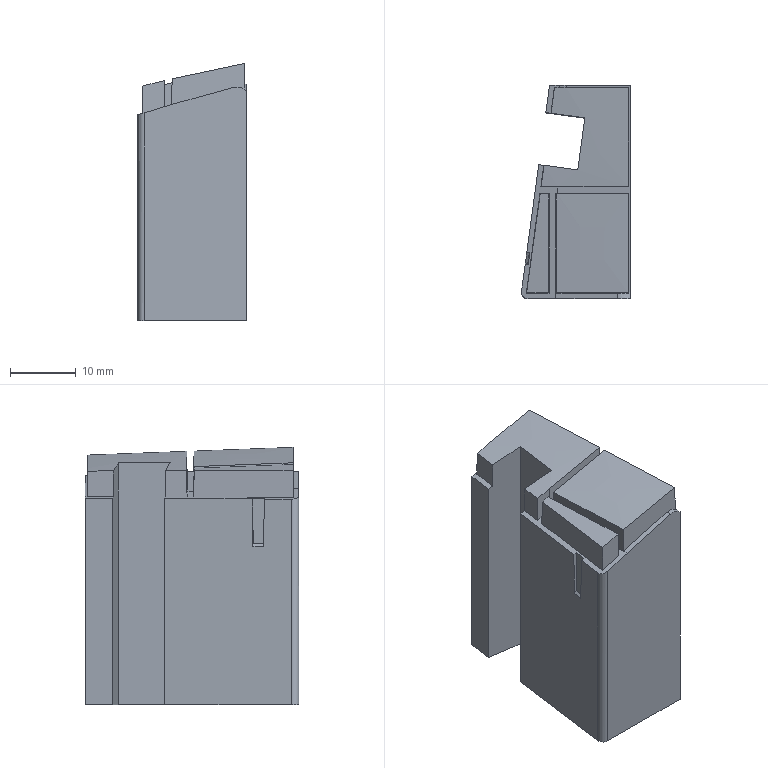Part | STEP file | P011002M012-000 | 1 solid | 76 faces | box 16.594 x 32.5 x 39.15 mm | volume 15176 mm3 | spline 34 | plane 23 | other 9 | cone 6 | cylinder 4 | commonest cylinder face diameters 2 x1 5 x1 5.98 x1 6 x1